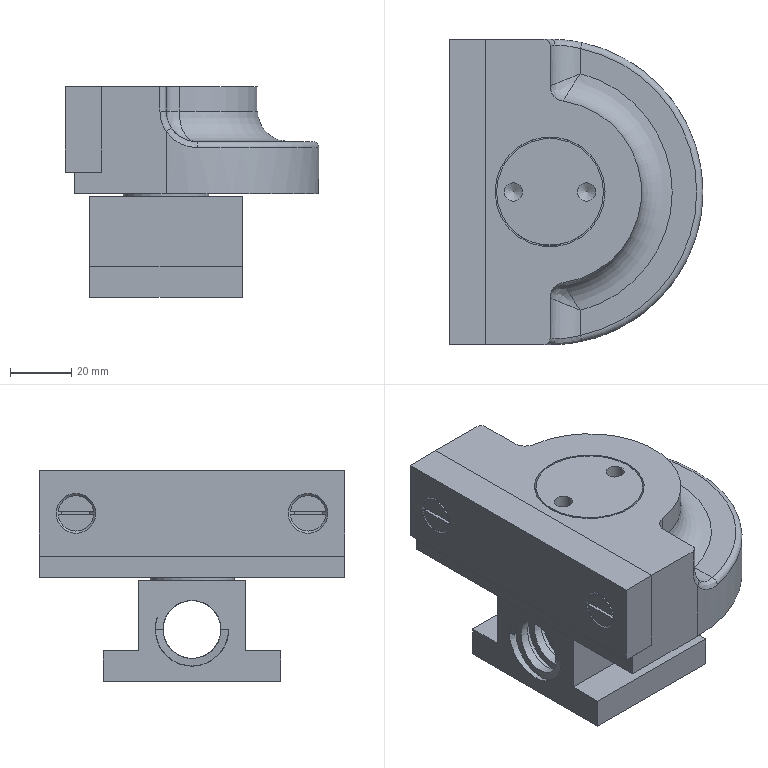Part | NX | features DATUM_CSYS 13, SKETCH 9, EXTRUDE 6, SIMPLE HOLE 6, HOLE PACKAGE 5, SYMBOLIC_THREAD 4, BLEND 3, CHAMFER 3, SWP104 3, BLOCK 2, CBORE_HOLE 1, CYLINDER 1, DATUM_ON_PATH 1, DELETE FACE 1, HELIX 1, SKIN 1, SUBTRACT 1, THREADS 1 | 6 solids | 129 faces | box 83 x 100 x 69 mm | volume 255059 mm3 | cylinder 52 | plane 48 | cone 15 | spline 10 | torus 4 | commonest cylinder face diameters 6 x26 5 x4 11.6 x4 4 x2 7 x2 10 x2